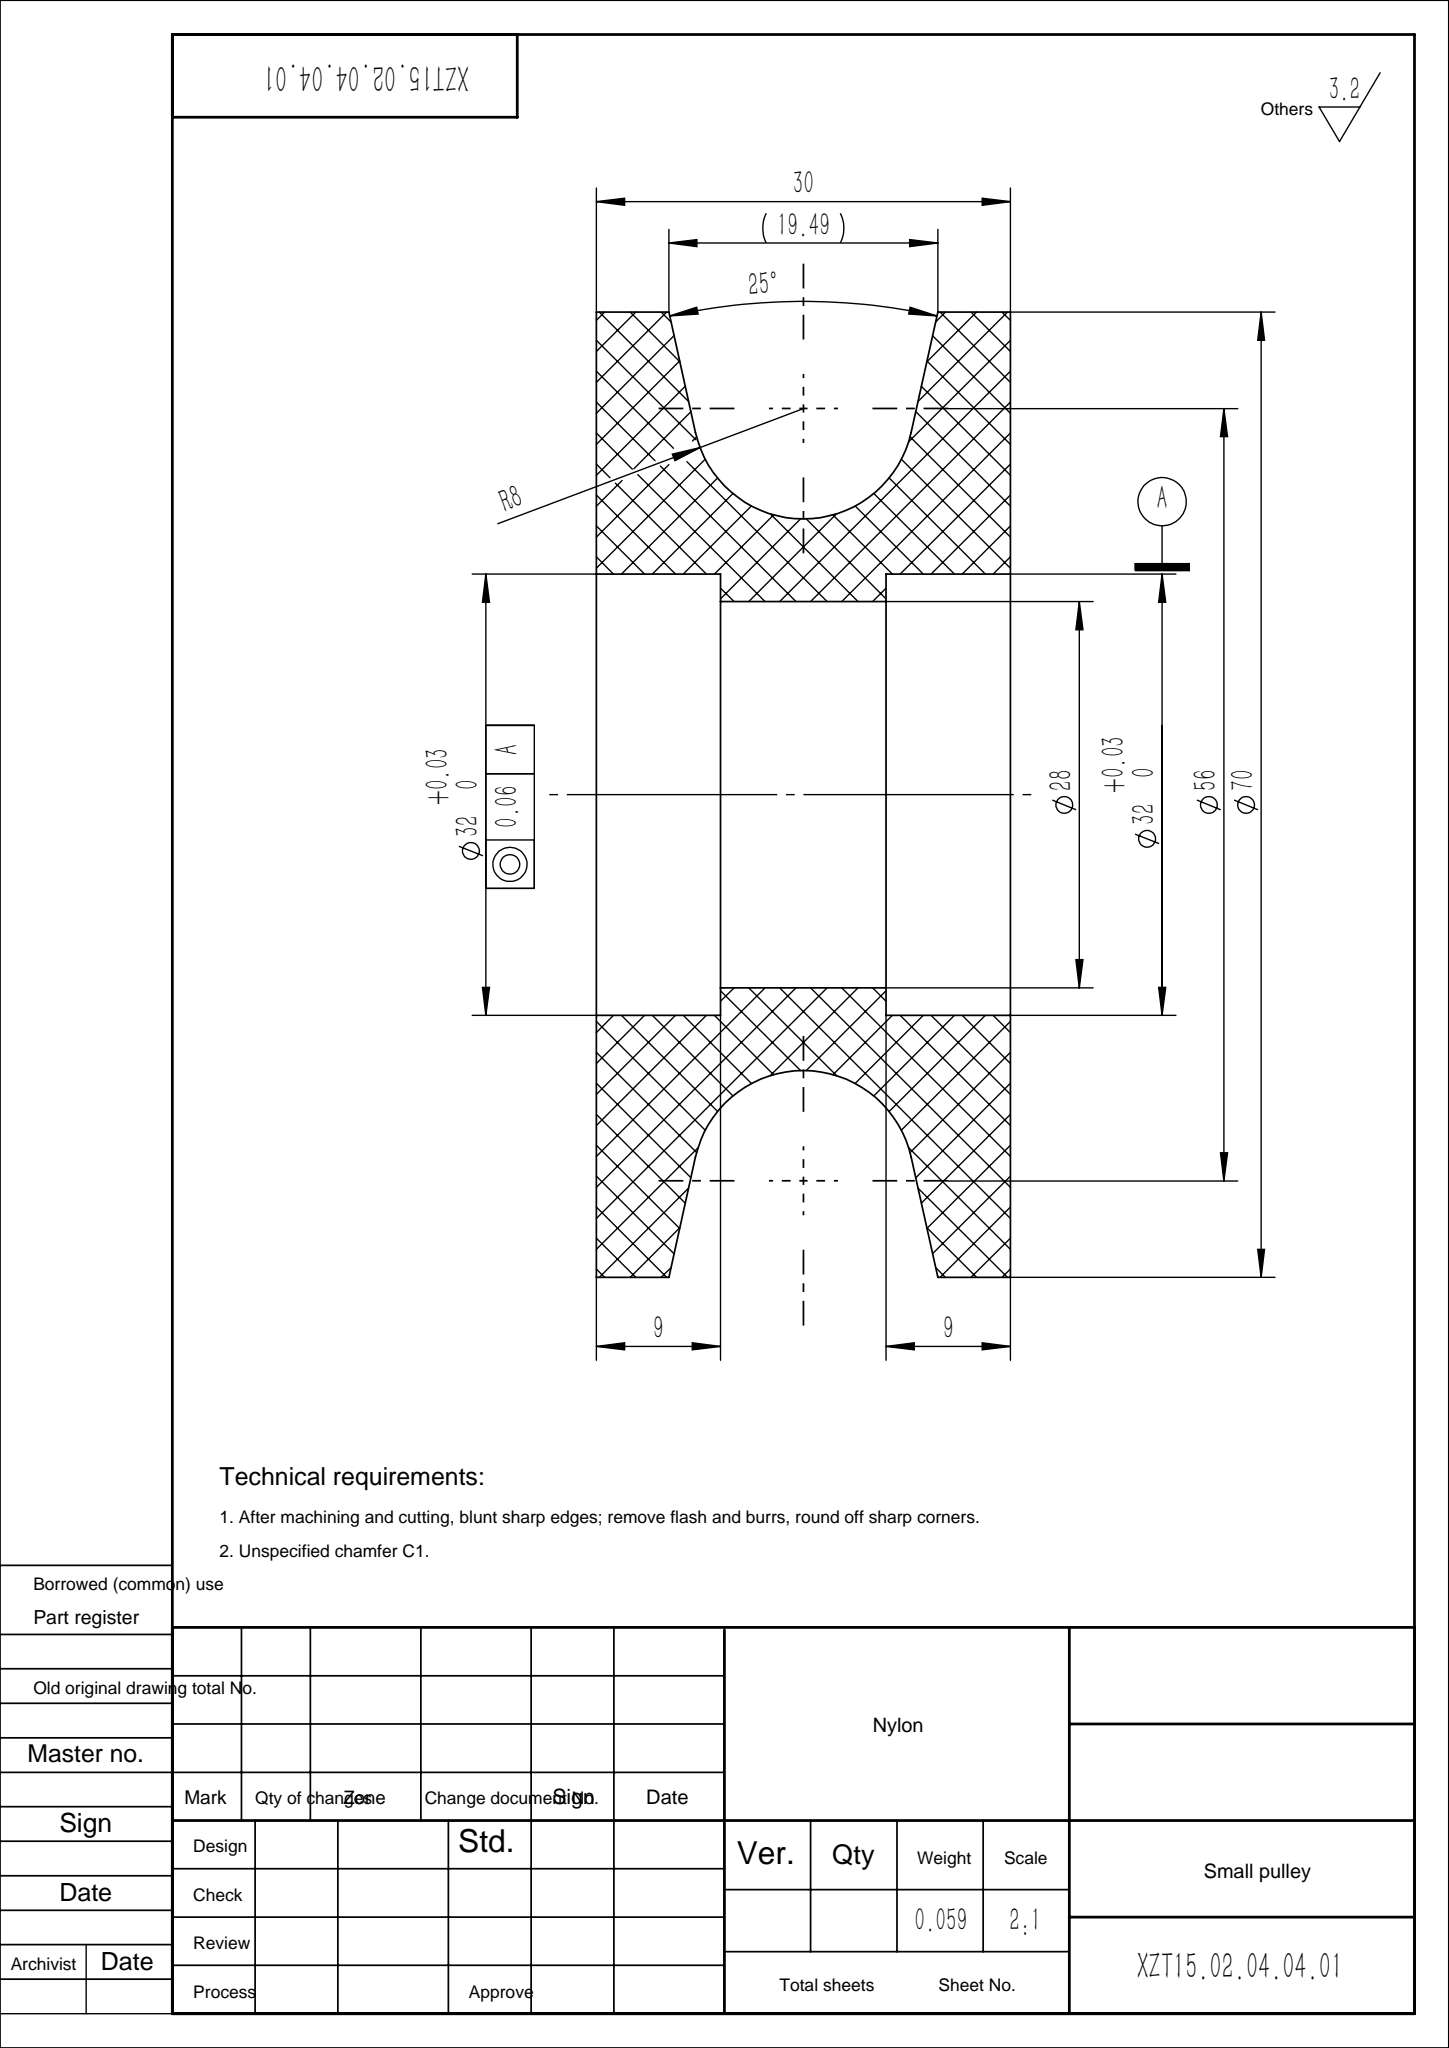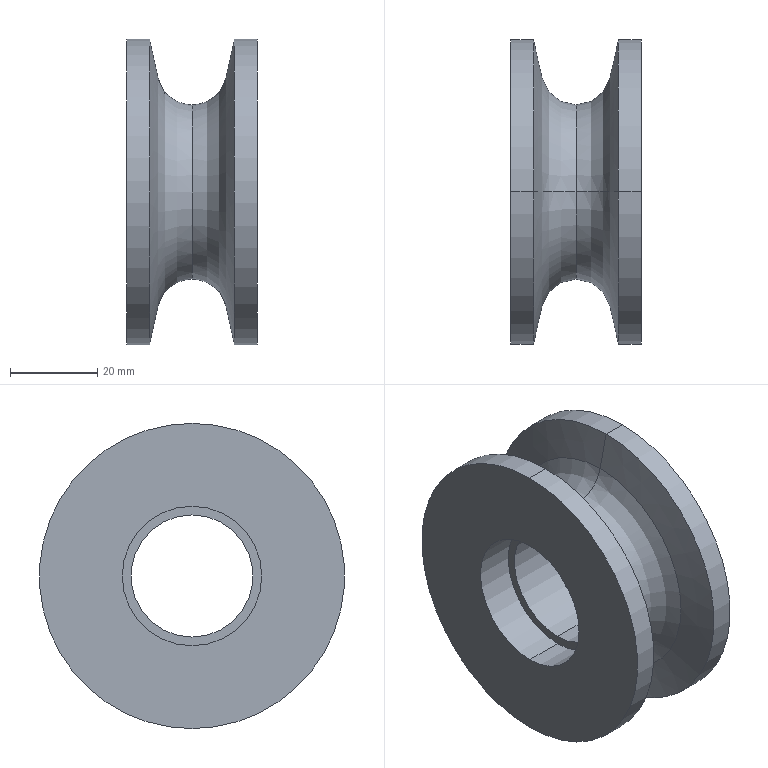Part | SolidWorks | features Revolution 1 | 1 solid | 22 faces | box 30 x 70 x 70 mm | volume 53072 mm3 | cylinder 10 | torus 4 | cone 4 | plane 4 | commonest cylinder face diameters 32 x4 70 x4 28 x2
STEP:
#1=CARTESIAN_POINT('',(-7.81,0.,26.268));
#2=VERTEX_POINT('',#1);
#3=CARTESIAN_POINT('',(0.,0.,20.));
#4=VERTEX_POINT('',#3);
#5=CARTESIAN_POINT('',(0.,0.,28.));
#6=DIRECTION('',(0.,-1.,0.));
#7=DIRECTION('',(0.,0.,-1.));
#8=AXIS2_PLACEMENT_3D('',#5,#6,#7);
#9=CIRCLE('',#8,8.);
#10=EDGE_CURVE('',#2,#4,#9,.T.);
#11=ORIENTED_EDGE('',*,*,#10,.T.);
#12=CARTESIAN_POINT('',(0.,0.,-20.));
#13=VERTEX_POINT('',#12);
#14=CARTESIAN_POINT('',(0.,0.,0.));
#15=DIRECTION('',(-1.,0.,0.));
#16=DIRECTION('',(0.,0.,1.));
#17=AXIS2_PLACEMENT_3D('',#14,#15,#16);
#18=CIRCLE('',#17,20.);
#19=EDGE_CURVE('',#4,#13,#18,.T.);
#20=ORIENTED_EDGE('',*,*,#19,.T.);
#21=CARTESIAN_POINT('',(-7.81,0.,-26.268));
#22=VERTEX_POINT('',#21);
#23=CARTESIAN_POINT('',(0.,0.,-28.));
#24=DIRECTION('',(0.,1.,0.));
#25=DIRECTION('',(0.,0.,1.));
#26=AXIS2_PLACEMENT_3D('',#23,#24,#25);
#27=CIRCLE('',#26,8.);
#28=EDGE_CURVE('',#22,#13,#27,.T.);
#29=ORIENTED_EDGE('',*,*,#28,.F.);
#30=CARTESIAN_POINT('',(-7.81,0.,0.));
#31=DIRECTION('',(-1.,0.,0.));
#32=DIRECTION('',(0.,0.,1.));
#33=AXIS2_PLACEMENT_3D('',#30,#31,#32);
#34=CIRCLE('',#33,26.268);
#35=EDGE_CURVE('',#2,#22,#34,.T.);
#36=ORIENTED_EDGE('',*,*,#35,.F.);
#37=EDGE_LOOP('',(#11,#20,#29,#36));
#38=FACE_OUTER_BOUND('',#37,.T.);
#39=CARTESIAN_POINT('',(0.,0.,0.));
#40=DIRECTION('',(-1.,0.,0.));
#41=DIRECTION('',(0.,0.,1.));
#42=AXIS2_PLACEMENT_3D('',#39,#40,#41);
#43=TOROIDAL_SURFACE('',#42,28.,8.);
#44=ADVANCED_FACE('',(#38),#43,.F.);
#45=ORIENTED_EDGE('',*,*,#28,.T.);
#46=CARTESIAN_POINT('',(0.,0.,0.));
#47=DIRECTION('',(-1.,0.,0.));
#48=DIRECTION('',(0.,0.,1.));
#49=AXIS2_PLACEMENT_3D('',#46,#47,#48);
#50=CIRCLE('',#49,20.);
#51=EDGE_CURVE('',#13,#4,#50,.T.);
#52=ORIENTED_EDGE('',*,*,#51,.T.);
#53=ORIENTED_EDGE('',*,*,#10,.F.);
#54=CARTESIAN_POINT('',(-7.81,0.,0.));
#55=DIRECTION('',(-1.,0.,0.));
#56=DIRECTION('',(0.,0.,1.));
#57=AXIS2_PLACEMENT_3D('',#54,#55,#56);
#58=CIRCLE('',#57,26.268);
#59=EDGE_CURVE('',#22,#2,#58,.T.);
#60=ORIENTED_EDGE('',*,*,#59,.F.);
#61=EDGE_LOOP('',(#45,#52,#53,#60));
#62=FACE_OUTER_BOUND('',#61,.T.);
#63=CARTESIAN_POINT('',(0.,0.,0.));
#64=DIRECTION('',(-1.,0.,0.));
#65=DIRECTION('',(0.,0.,1.));
#66=AXIS2_PLACEMENT_3D('',#63,#64,#65);
#67=TOROIDAL_SURFACE('',#66,28.,8.);
#68=ADVANCED_FACE('',(#62),#67,.F.);
#69=CARTESIAN_POINT('',(15.,0.,-16.));
#70=VERTEX_POINT('',#69);
#71=CARTESIAN_POINT('',(15.,0.,16.));
#72=VERTEX_POINT('',#71);
#73=CARTESIAN_POINT('',(15.,0.,0.));
#74=DIRECTION('',(-1.,0.,0.));
#75=DIRECTION('',(0.,0.,1.));
#76=AXIS2_PLACEMENT_3D('',#73,#74,#75);
#77=CIRCLE('',#76,16.);
#78=EDGE_CURVE('',#70,#72,#77,.T.);
#79=ORIENTED_EDGE('',*,*,#78,.F.);
#80=CARTESIAN_POINT('',(6.,0.,-16.));
#81=VERTEX_POINT('',#80);
#82=CARTESIAN_POINT('',(0.,0.,-16.));
#83=DIRECTION('',(-1.,0.,0.));
#84=VECTOR('',#83,1000.);
#85=LINE('',#82,#84);
#86=EDGE_CURVE('',#70,#81,#85,.T.);
#87=ORIENTED_EDGE('',*,*,#86,.T.);
#88=CARTESIAN_POINT('',(6.,0.,16.));
#89=VERTEX_POINT('',#88);
#90=CARTESIAN_POINT('',(6.,0.,0.));
#91=DIRECTION('',(-1.,0.,0.));
#92=DIRECTION('',(0.,0.,1.));
#93=AXIS2_PLACEMENT_3D('',#90,#91,#92);
#94=CIRCLE('',#93,16.);
#95=EDGE_CURVE('',#81,#89,#94,.T.);
#96=ORIENTED_EDGE('',*,*,#95,.T.);
#97=CARTESIAN_POINT('',(0.,0.,16.));
#98=DIRECTION('',(-1.,0.,0.));
#99=VECTOR('',#98,1000.);
#100=LINE('',#97,#99);
#101=EDGE_CURVE('',#72,#89,#100,.T.);
#102=ORIENTED_EDGE('',*,*,#101,.F.);
#103=EDGE_LOOP('',(#79,#87,#96,#102));
#104=FACE_OUTER_BOUND('',#103,.T.);
#105=CARTESIAN_POINT('',(0.,0.,0.));
#106=DIRECTION('',(-1.,0.,0.));
#107=DIRECTION('',(0.,0.,1.));
#108=AXIS2_PLACEMENT_3D('',#105,#106,#107);
#109=CYLINDRICAL_SURFACE('',#108,16.);
#110=ADVANCED_FACE('',(#104),#109,.F.);
#111=CARTESIAN_POINT('',(15.,0.,35.));
#112=VERTEX_POINT('',#111);
#113=CARTESIAN_POINT('',(15.,0.,-35.));
#114=VERTEX_POINT('',#113);
#115=CARTESIAN_POINT('',(15.,0.,0.));
#116=DIRECTION('',(-1.,0.,0.));
#117=DIRECTION('',(0.,0.,1.));
#118=AXIS2_PLACEMENT_3D('',#115,#116,#117);
#119=CIRCLE('',#118,35.);
#120=EDGE_CURVE('',#112,#114,#119,.T.);
#121=ORIENTED_EDGE('',*,*,#120,.T.);
#122=CARTESIAN_POINT('',(9.746,0.,-35.));
#123=VERTEX_POINT('',#122);
#124=CARTESIAN_POINT('',(0.,0.,-35.));
#125=DIRECTION('',(-1.,0.,0.));
#126=VECTOR('',#125,1000.);
#127=LINE('',#124,#126);
#128=EDGE_CURVE('',#114,#123,#127,.T.);
#129=ORIENTED_EDGE('',*,*,#128,.T.);
#130=CARTESIAN_POINT('',(9.746,0.,35.));
#131=VERTEX_POINT('',#130);
#132=CARTESIAN_POINT('',(9.746,0.,0.));
#133=DIRECTION('',(-1.,0.,0.));
#134=DIRECTION('',(0.,0.,1.));
#135=AXIS2_PLACEMENT_3D('',#132,#133,#134);
#136=CIRCLE('',#135,35.);
#137=EDGE_CURVE('',#131,#123,#136,.T.);
#138=ORIENTED_EDGE('',*,*,#137,.F.);
#139=CARTESIAN_POINT('',(0.,0.,35.));
#140=DIRECTION('',(-1.,0.,0.));
#141=VECTOR('',#140,1000.);
#142=LINE('',#139,#141);
#143=EDGE_CURVE('',#112,#131,#142,.T.);
#144=ORIENTED_EDGE('',*,*,#143,.F.);
#145=EDGE_LOOP('',(#121,#129,#138,#144));
#146=FACE_OUTER_BOUND('',#145,.T.);
#147=CARTESIAN_POINT('',(0.,0.,0.));
#148=DIRECTION('',(-1.,0.,0.));
#149=DIRECTION('',(0.,0.,1.));
#150=AXIS2_PLACEMENT_3D('',#147,#148,#149);
#151=CYLINDRICAL_SURFACE('',#150,35.);
#152=ADVANCED_FACE('',(#146),#151,.T.);
#153=CARTESIAN_POINT('',(7.81,0.,26.268));
#154=VERTEX_POINT('',#153);
#155=CARTESIAN_POINT('',(7.81,0.,-26.268));
#156=VERTEX_POINT('',#155);
#157=CARTESIAN_POINT('',(7.81,0.,0.));
#158=DIRECTION('',(-1.,0.,0.));
#159=DIRECTION('',(0.,0.,1.));
#160=AXIS2_PLACEMENT_3D('',#157,#158,#159);
#161=CIRCLE('',#160,26.268);
#162=EDGE_CURVE('',#154,#156,#161,.T.);
#163=ORIENTED_EDGE('',*,*,#162,.F.);
#164=CARTESIAN_POINT('',(9.746,0.,35.));
#165=DIRECTION('',(0.2164,0.,0.9763));
#166=VECTOR('',#165,1000.);
#167=LINE('',#164,#166);
#168=EDGE_CURVE('',#154,#131,#167,.T.);
#169=ORIENTED_EDGE('',*,*,#168,.T.);
#170=ORIENTED_EDGE('',*,*,#137,.T.);
#171=CARTESIAN_POINT('',(9.746,0.,-35.));
#172=DIRECTION('',(0.2164,0.,-0.9763));
#173=VECTOR('',#172,1000.);
#174=LINE('',#171,#173);
#175=EDGE_CURVE('',#156,#123,#174,.T.);
#176=ORIENTED_EDGE('',*,*,#175,.F.);
#177=EDGE_LOOP('',(#163,#169,#170,#176));
#178=FACE_OUTER_BOUND('',#177,.T.);
#179=CARTESIAN_POINT('',(9.746,0.,0.));
#180=DIRECTION('',(1.,0.,0.));
#181=DIRECTION('',(0.,0.,-1.));
#182=AXIS2_PLACEMENT_3D('',#179,#180,#181);
#183=CONICAL_SURFACE('',#182,35.,1.353);
#184=ADVANCED_FACE('',(#178),#183,.T.);
#185=ORIENTED_EDGE('',*,*,#51,.F.);
#186=CARTESIAN_POINT('',(0.,0.,-28.));
#187=DIRECTION('',(0.,1.,0.));
#188=DIRECTION('',(0.,0.,1.));
#189=AXIS2_PLACEMENT_3D('',#186,#187,#188);
#190=CIRCLE('',#189,8.);
#191=EDGE_CURVE('',#13,#156,#190,.T.);
#192=ORIENTED_EDGE('',*,*,#191,.T.);
#193=CARTESIAN_POINT('',(7.81,0.,0.));
#194=DIRECTION('',(-1.,0.,0.));
#195=DIRECTION('',(0.,0.,1.));
#196=AXIS2_PLACEMENT_3D('',#193,#194,#195);
#197=CIRCLE('',#196,26.268);
#198=EDGE_CURVE('',#156,#154,#197,.T.);
#199=ORIENTED_EDGE('',*,*,#198,.T.);
#200=CARTESIAN_POINT('',(0.,0.,28.));
#201=DIRECTION('',(0.,-1.,0.));
#202=DIRECTION('',(0.,0.,-1.));
#203=AXIS2_PLACEMENT_3D('',#200,#201,#202);
#204=CIRCLE('',#203,8.);
#205=EDGE_CURVE('',#4,#154,#204,.T.);
#206=ORIENTED_EDGE('',*,*,#205,.F.);
#207=EDGE_LOOP('',(#185,#192,#199,#206));
#208=FACE_OUTER_BOUND('',#207,.T.);
#209=CARTESIAN_POINT('',(0.,0.,0.));
#210=DIRECTION('',(-1.,0.,0.));
#211=DIRECTION('',(0.,0.,1.));
#212=AXIS2_PLACEMENT_3D('',#209,#210,#211);
#213=TOROIDAL_SURFACE('',#212,28.,8.);
#214=ADVANCED_FACE('',(#208),#213,.F.);
#215=ORIENTED_EDGE('',*,*,#35,.T.);
#216=CARTESIAN_POINT('',(-9.746,0.,-35.));
#217=VERTEX_POINT('',#216);
#218=CARTESIAN_POINT('',(-7.81,0.,-26.268));
#219=DIRECTION('',(-0.2164,0.,-0.9763));
#220=VECTOR('',#219,1000.);
#221=LINE('',#218,#220);
#222=EDGE_CURVE('',#22,#217,#221,.T.);
#223=ORIENTED_EDGE('',*,*,#222,.T.);
#224=CARTESIAN_POINT('',(-9.746,0.,35.));
#225=VERTEX_POINT('',#224);
#226=CARTESIAN_POINT('',(-9.746,0.,0.));
#227=DIRECTION('',(-1.,0.,0.));
#228=DIRECTION('',(0.,0.,1.));
#229=AXIS2_PLACEMENT_3D('',#226,#227,#228);
#230=CIRCLE('',#229,35.);
#231=EDGE_CURVE('',#225,#217,#230,.T.);
#232=ORIENTED_EDGE('',*,*,#231,.F.);
#233=CARTESIAN_POINT('',(-7.81,0.,26.268));
#234=DIRECTION('',(-0.2164,0.,0.9763));
#235=VECTOR('',#234,1000.);
#236=LINE('',#233,#235);
#237=EDGE_CURVE('',#2,#225,#236,.T.);
#238=ORIENTED_EDGE('',*,*,#237,.F.);
#239=EDGE_LOOP('',(#215,#223,#232,#238));
#240=FACE_OUTER_BOUND('',#239,.T.);
#241=CARTESIAN_POINT('',(-7.81,0.,0.));
#242=DIRECTION('',(-1.,0.,0.));
#243=DIRECTION('',(0.,0.,1.));
#244=AXIS2_PLACEMENT_3D('',#241,#242,#243);
#245=CONICAL_SURFACE('',#244,26.268,1.353);
#246=ADVANCED_FACE('',(#240),#245,.T.);
#247=ORIENTED_EDGE('',*,*,#231,.T.);
#248=CARTESIAN_POINT('',(-15.,0.,-35.));
#249=VERTEX_POINT('',#248);
#250=CARTESIAN_POINT('',(0.,0.,-35.));
#251=DIRECTION('',(-1.,0.,0.));
#252=VECTOR('',#251,1000.);
#253=LINE('',#250,#252);
#254=EDGE_CURVE('',#217,#249,#253,.T.);
#255=ORIENTED_EDGE('',*,*,#254,.T.);
#256=CARTESIAN_POINT('',(-15.,0.,35.));
#257=VERTEX_POINT('',#256);
#258=CARTESIAN_POINT('',(-15.,0.,0.));
#259=DIRECTION('',(-1.,0.,0.));
#260=DIRECTION('',(0.,0.,1.));
#261=AXIS2_PLACEMENT_3D('',#258,#259,#260);
#262=CIRCLE('',#261,35.);
#263=EDGE_CURVE('',#257,#249,#262,.T.);
#264=ORIENTED_EDGE('',*,*,#263,.F.);
#265=CARTESIAN_POINT('',(0.,0.,35.));
#266=DIRECTION('',(-1.,0.,0.));
#267=VECTOR('',#266,1000.);
#268=LINE('',#265,#267);
#269=EDGE_CURVE('',#225,#257,#268,.T.);
#270=ORIENTED_EDGE('',*,*,#269,.F.);
#271=EDGE_LOOP('',(#247,#255,#264,#270));
#272=FACE_OUTER_BOUND('',#271,.T.);
#273=CARTESIAN_POINT('',(0.,0.,0.));
#274=DIRECTION('',(-1.,0.,0.));
#275=DIRECTION('',(0.,0.,1.));
#276=AXIS2_PLACEMENT_3D('',#273,#274,#275);
#277=CYLINDRICAL_SURFACE('',#276,35.);
#278=ADVANCED_FACE('',(#272),#277,.T.);
#279=CARTESIAN_POINT('',(-6.,0.,-16.));
#280=VERTEX_POINT('',#279);
#281=CARTESIAN_POINT('',(-6.,0.,16.));
#282=VERTEX_POINT('',#281);
#283=CARTESIAN_POINT('',(-6.,0.,0.));
#284=DIRECTION('',(-1.,0.,0.));
#285=DIRECTION('',(0.,0.,1.));
#286=AXIS2_PLACEMENT_3D('',#283,#284,#285);
#287=CIRCLE('',#286,16.);
#288=EDGE_CURVE('',#280,#282,#287,.T.);
#289=ORIENTED_EDGE('',*,*,#288,.F.);
#290=CARTESIAN_POINT('',(-15.,0.,-16.));
#291=VERTEX_POINT('',#290);
#292=CARTESIAN_POINT('',(0.,0.,-16.));
#293=DIRECTION('',(-1.,0.,0.));
#294=VECTOR('',#293,1000.);
#295=LINE('',#292,#294);
#296=EDGE_CURVE('',#280,#291,#295,.T.);
#297=ORIENTED_EDGE('',*,*,#296,.T.);
#298=CARTESIAN_POINT('',(-15.,0.,16.));
#299=VERTEX_POINT('',#298);
#300=CARTESIAN_POINT('',(-15.,0.,0.));
#301=DIRECTION('',(-1.,0.,0.));
#302=DIRECTION('',(0.,0.,1.));
#303=AXIS2_PLACEMENT_3D('',#300,#301,#302);
#304=CIRCLE('',#303,16.);
#305=EDGE_CURVE('',#291,#299,#304,.T.);
#306=ORIENTED_EDGE('',*,*,#305,.T.);
#307=CARTESIAN_POINT('',(0.,0.,16.));
#308=DIRECTION('',(-1.,0.,0.));
#309=VECTOR('',#308,1000.);
#310=LINE('',#307,#309);
#311=EDGE_CURVE('',#282,#299,#310,.T.);
#312=ORIENTED_EDGE('',*,*,#311,.F.);
#313=EDGE_LOOP('',(#289,#297,#306,#312));
#314=FACE_OUTER_BOUND('',#313,.T.);
#315=CARTESIAN_POINT('',(0.,0.,0.));
#316=DIRECTION('',(-1.,0.,0.));
#317=DIRECTION('',(0.,0.,1.));
#318=AXIS2_PLACEMENT_3D('',#315,#316,#317);
#319=CYLINDRICAL_SURFACE('',#318,16.);
#320=ADVANCED_FACE('',(#314),#319,.F.);
#321=CARTESIAN_POINT('',(6.,0.,-14.));
#322=VERTEX_POINT('',#321);
#323=CARTESIAN_POINT('',(6.,0.,14.));
#324=VERTEX_POINT('',#323);
#325=CARTESIAN_POINT('',(6.,0.,0.));
#326=DIRECTION('',(-1.,0.,0.));
#327=DIRECTION('',(0.,0.,1.));
#328=AXIS2_PLACEMENT_3D('',#325,#326,#327);
#329=CIRCLE('',#328,14.);
#330=EDGE_CURVE('',#322,#324,#329,.T.);
#331=ORIENTED_EDGE('',*,*,#330,.F.);
#332=CARTESIAN_POINT('',(-6.,0.,-14.));
#333=VERTEX_POINT('',#332);
#334=CARTESIAN_POINT('',(0.,0.,-14.));
#335=DIRECTION('',(-1.,0.,0.));
#336=VECTOR('',#335,1000.);
#337=LINE('',#334,#336);
#338=EDGE_CURVE('',#322,#333,#337,.T.);
#339=ORIENTED_EDGE('',*,*,#338,.T.);
#340=CARTESIAN_POINT('',(-6.,0.,14.));
#341=VERTEX_POINT('',#340);
#342=CARTESIAN_POINT('',(-6.,0.,0.));
#343=DIRECTION('',(-1.,0.,0.));
#344=DIRECTION('',(0.,0.,1.));
#345=AXIS2_PLACEMENT_3D('',#342,#343,#344);
#346=CIRCLE('',#345,14.);
#347=EDGE_CURVE('',#333,#341,#346,.T.);
#348=ORIENTED_EDGE('',*,*,#347,.T.);
#349=CARTESIAN_POINT('',(0.,0.,14.));
#350=DIRECTION('',(-1.,0.,0.));
#351=VECTOR('',#350,1000.);
#352=LINE('',#349,#351);
#353=EDGE_CURVE('',#324,#341,#352,.T.);
#354=ORIENTED_EDGE('',*,*,#353,.F.);
#355=EDGE_LOOP('',(#331,#339,#348,#354));
#356=FACE_OUTER_BOUND('',#355,.T.);
#357=CARTESIAN_POINT('',(0.,0.,0.));
#358=DIRECTION('',(-1.,0.,0.));
#359=DIRECTION('',(0.,0.,1.));
#360=AXIS2_PLACEMENT_3D('',#357,#358,#359);
#361=CYLINDRICAL_SURFACE('',#360,14.);
#362=ADVANCED_FACE('',(#356),#361,.F.);
#363=CARTESIAN_POINT('',(6.,0.,0.));
#364=DIRECTION('',(-1.,0.,0.));
#365=DIRECTION('',(0.,0.,1.));
#366=AXIS2_PLACEMENT_3D('',#363,#364,#365);
#367=CIRCLE('',#366,16.);
#368=EDGE_CURVE('',#89,#81,#367,.T.);
#369=ORIENTED_EDGE('',*,*,#368,.F.);
#370=ORIENTED_EDGE('',*,*,#95,.F.);
#371=EDGE_LOOP('',(#369,#370));
#372=FACE_OUTER_BOUND('',#371,.T.);
#373=CARTESIAN_POINT('',(6.,0.,0.));
#374=DIRECTION('',(-1.,0.,0.));
#375=DIRECTION('',(0.,0.,1.));
#376=AXIS2_PLACEMENT_3D('',#373,#374,#375);
#377=CIRCLE('',#376,14.);
#378=EDGE_CURVE('',#324,#322,#377,.T.);
#379=ORIENTED_EDGE('',*,*,#378,.T.);
#380=ORIENTED_EDGE('',*,*,#330,.T.);
#381=EDGE_LOOP('',(#379,#380));
#382=FACE_BOUND('',#381,.T.);
#383=CARTESIAN_POINT('',(6.,14.,0.));
#384=DIRECTION('',(-1.,0.,0.));
#385=DIRECTION('',(0.,0.,1.));
#386=AXIS2_PLACEMENT_3D('',#383,#384,#385);
#387=PLANE('',#386);
#388=ADVANCED_FACE('',(#372,#382),#387,.F.);
#389=ORIENTED_EDGE('',*,*,#338,.F.);
#390=ORIENTED_EDGE('',*,*,#378,.F.);
#391=ORIENTED_EDGE('',*,*,#353,.T.);
#392=CARTESIAN_POINT('',(-6.,0.,0.));
#393=DIRECTION('',(-1.,0.,0.));
#394=DIRECTION('',(0.,0.,1.));
#395=AXIS2_PLACEMENT_3D('',#392,#393,#394);
#396=CIRCLE('',#395,14.);
#397=EDGE_CURVE('',#341,#333,#396,.T.);
#398=ORIENTED_EDGE('',*,*,#397,.T.);
#399=EDGE_LOOP('',(#389,#390,#391,#398));
#400=FACE_OUTER_BOUND('',#399,.T.);
#401=CARTESIAN_POINT('',(0.,0.,0.));
#402=DIRECTION('',(-1.,0.,0.));
#403=DIRECTION('',(0.,0.,1.));
#404=AXIS2_PLACEMENT_3D('',#401,#402,#403);
#405=CYLINDRICAL_SURFACE('',#404,14.);
#406=ADVANCED_FACE('',(#400),#405,.F.);
#407=ORIENTED_EDGE('',*,*,#397,.F.);
#408=ORIENTED_EDGE('',*,*,#347,.F.);
#409=EDGE_LOOP('',(#407,#408));
#410=FACE_BOUND('',#409,.T.);
#411=CARTESIAN_POINT('',(-6.,0.,0.));
#412=DIRECTION('',(-1.,0.,0.));
#413=DIRECTION('',(0.,0.,1.));
#414=AXIS2_PLACEMENT_3D('',#411,#412,#413);
#415=CIRCLE('',#414,16.);
#416=EDGE_CURVE('',#282,#280,#415,.T.);
#417=ORIENTED_EDGE('',*,*,#416,.T.);
#418=ORIENTED_EDGE('',*,*,#288,.T.);
#419=EDGE_LOOP('',(#417,#418));
#420=FACE_OUTER_BOUND('',#419,.T.);
#421=CARTESIAN_POINT('',(-6.,14.,0.));
#422=DIRECTION('',(1.,0.,0.));
#423=DIRECTION('',(0.,0.,-1.));
#424=AXIS2_PLACEMENT_3D('',#421,#422,#423);
#425=PLANE('',#424);
#426=ADVANCED_FACE('',(#410,#420),#425,.F.);
#427=ORIENTED_EDGE('',*,*,#296,.F.);
#428=ORIENTED_EDGE('',*,*,#416,.F.);
#429=ORIENTED_EDGE('',*,*,#311,.T.);
#430=CARTESIAN_POINT('',(-15.,0.,0.));
#431=DIRECTION('',(-1.,0.,0.));
#432=DIRECTION('',(0.,0.,1.));
#433=AXIS2_PLACEMENT_3D('',#430,#431,#432);
#434=CIRCLE('',#433,16.);
#435=EDGE_CURVE('',#299,#291,#434,.T.);
#436=ORIENTED_EDGE('',*,*,#435,.T.);
#437=EDGE_LOOP('',(#427,#428,#429,#436));
#438=FACE_OUTER_BOUND('',#437,.T.);
#439=CARTESIAN_POINT('',(0.,0.,0.));
#440=DIRECTION('',(-1.,0.,0.));
#441=DIRECTION('',(0.,0.,1.));
#442=AXIS2_PLACEMENT_3D('',#439,#440,#441);
#443=CYLINDRICAL_SURFACE('',#442,16.);
#444=ADVANCED_FACE('',(#438),#443,.F.);
#445=ORIENTED_EDGE('',*,*,#435,.F.);
#446=ORIENTED_EDGE('',*,*,#305,.F.);
#447=EDGE_LOOP('',(#445,#446));
#448=FACE_BOUND('',#447,.T.);
#449=ORIENTED_EDGE('',*,*,#263,.T.);
#450=CARTESIAN_POINT('',(-15.,0.,0.));
#451=DIRECTION('',(-1.,0.,0.));
#452=DIRECTION('',(0.,0.,1.));
#453=AXIS2_PLACEMENT_3D('',#450,#451,#452);
#454=CIRCLE('',#453,35.);
#455=EDGE_CURVE('',#249,#257,#454,.T.);
#456=ORIENTED_EDGE('',*,*,#455,.T.);
#457=EDGE_LOOP('',(#449,#456));
#458=FACE_OUTER_BOUND('',#457,.T.);
#459=CARTESIAN_POINT('',(-15.,16.,0.));
#460=DIRECTION('',(1.,0.,0.));
#461=DIRECTION('',(0.,0.,-1.));
#462=AXIS2_PLACEMENT_3D('',#459,#460,#461);
#463=PLANE('',#462);
#464=ADVANCED_FACE('',(#448,#458),#463,.F.);
#465=ORIENTED_EDGE('',*,*,#254,.F.);
#466=CARTESIAN_POINT('',(-9.746,0.,0.));
#467=DIRECTION('',(-1.,0.,0.));
#468=DIRECTION('',(0.,0.,1.));
#469=AXIS2_PLACEMENT_3D('',#466,#467,#468);
#470=CIRCLE('',#469,35.);
#471=EDGE_CURVE('',#217,#225,#470,.T.);
#472=ORIENTED_EDGE('',*,*,#471,.T.);
#473=ORIENTED_EDGE('',*,*,#269,.T.);
#474=ORIENTED_EDGE('',*,*,#455,.F.);
#475=EDGE_LOOP('',(#465,#472,#473,#474));
#476=FACE_OUTER_BOUND('',#475,.T.);
#477=CARTESIAN_POINT('',(0.,0.,0.));
#478=DIRECTION('',(-1.,0.,0.));
#479=DIRECTION('',(0.,0.,1.));
#480=AXIS2_PLACEMENT_3D('',#477,#478,#479);
#481=CYLINDRICAL_SURFACE('',#480,35.);
#482=ADVANCED_FACE('',(#476),#481,.T.);
#483=ORIENTED_EDGE('',*,*,#222,.F.);
#484=ORIENTED_EDGE('',*,*,#59,.T.);
#485=ORIENTED_EDGE('',*,*,#237,.T.);
#486=ORIENTED_EDGE('',*,*,#471,.F.);
#487=EDGE_LOOP('',(#483,#484,#485,#486));
#488=FACE_OUTER_BOUND('',#487,.T.);
#489=CARTESIAN_POINT('',(-7.81,0.,0.));
#490=DIRECTION('',(-1.,0.,0.));
#491=DIRECTION('',(0.,0.,1.));
#492=AXIS2_PLACEMENT_3D('',#489,#490,#491);
#493=CONICAL_SURFACE('',#492,26.268,1.353);
#494=ADVANCED_FACE('',(#488),#493,.T.);
#495=ORIENTED_EDGE('',*,*,#19,.F.);
#496=ORIENTED_EDGE('',*,*,#205,.T.);
#497=ORIENTED_EDGE('',*,*,#162,.T.);
#498=ORIENTED_EDGE('',*,*,#191,.F.);
#499=EDGE_LOOP('',(#495,#496,#497,#498));
#500=FACE_OUTER_BOUND('',#499,.T.);
#501=CARTESIAN_POINT('',(0.,0.,0.));
#502=DIRECTION('',(-1.,0.,0.));
#503=DIRECTION('',(0.,0.,1.));
#504=AXIS2_PLACEMENT_3D('',#501,#502,#503);
#505=TOROIDAL_SURFACE('',#504,28.,8.);
#506=ADVANCED_FACE('',(#500),#505,.F.);
#507=ORIENTED_EDGE('',*,*,#168,.F.);
#508=ORIENTED_EDGE('',*,*,#198,.F.);
#509=ORIENTED_EDGE('',*,*,#175,.T.);
#510=CARTESIAN_POINT('',(9.746,0.,0.));
#511=DIRECTION('',(-1.,0.,0.));
#512=DIRECTION('',(0.,0.,1.));
#513=AXIS2_PLACEMENT_3D('',#510,#511,#512);
#514=CIRCLE('',#513,35.);
#515=EDGE_CURVE('',#123,#131,#514,.T.);
#516=ORIENTED_EDGE('',*,*,#515,.T.);
#517=EDGE_LOOP('',(#507,#508,#509,#516));
#518=FACE_OUTER_BOUND('',#517,.T.);
#519=CARTESIAN_POINT('',(9.746,0.,0.));
#520=DIRECTION('',(1.,0.,0.));
#521=DIRECTION('',(0.,0.,-1.));
#522=AXIS2_PLACEMENT_3D('',#519,#520,#521);
#523=CONICAL_SURFACE('',#522,35.,1.353);
#524=ADVANCED_FACE('',(#518),#523,.T.);
#525=ORIENTED_EDGE('',*,*,#128,.F.);
#526=CARTESIAN_POINT('',(15.,0.,0.));
#527=DIRECTION('',(-1.,0.,0.));
#528=DIRECTION('',(0.,0.,1.));
#529=AXIS2_PLACEMENT_3D('',#526,#527,#528);
#530=CIRCLE('',#529,35.);
#531=EDGE_CURVE('',#114,#112,#530,.T.);
#532=ORIENTED_EDGE('',*,*,#531,.T.);
#533=ORIENTED_EDGE('',*,*,#143,.T.);
#534=ORIENTED_EDGE('',*,*,#515,.F.);
#535=EDGE_LOOP('',(#525,#532,#533,#534));
#536=FACE_OUTER_BOUND('',#535,.T.);
#537=CARTESIAN_POINT('',(0.,0.,0.));
#538=DIRECTION('',(-1.,0.,0.));
#539=DIRECTION('',(0.,0.,1.));
#540=AXIS2_PLACEMENT_3D('',#537,#538,#539);
#541=CYLINDRICAL_SURFACE('',#540,35.);
#542=ADVANCED_FACE('',(#536),#541,.T.);
#543=ORIENTED_EDGE('',*,*,#120,.F.);
#544=ORIENTED_EDGE('',*,*,#531,.F.);
#545=EDGE_LOOP('',(#543,#544));
#546=FACE_OUTER_BOUND('',#545,.T.);
#547=CARTESIAN_POINT('',(15.,0.,0.));
#548=DIRECTION('',(-1.,0.,0.));
#549=DIRECTION('',(0.,0.,1.));
#550=AXIS2_PLACEMENT_3D('',#547,#548,#549);
#551=CIRCLE('',#550,16.);
#552=EDGE_CURVE('',#72,#70,#551,.T.);
#553=ORIENTED_EDGE('',*,*,#552,.T.);
#554=ORIENTED_EDGE('',*,*,#78,.T.);
#555=EDGE_LOOP('',(#553,#554));
#556=FACE_BOUND('',#555,.T.);
#557=CARTESIAN_POINT('',(15.,16.,0.));
#558=DIRECTION('',(-1.,0.,0.));
#559=DIRECTION('',(0.,0.,1.));
#560=AXIS2_PLACEMENT_3D('',#557,#558,#559);
#561=PLANE('',#560);
#562=ADVANCED_FACE('',(#546,#556),#561,.F.);
#563=ORIENTED_EDGE('',*,*,#86,.F.);
#564=ORIENTED_EDGE('',*,*,#552,.F.);
#565=ORIENTED_EDGE('',*,*,#101,.T.);
#566=ORIENTED_EDGE('',*,*,#368,.T.);
#567=EDGE_LOOP('',(#563,#564,#565,#566));
#568=FACE_OUTER_BOUND('',#567,.T.);
#569=CARTESIAN_POINT('',(0.,0.,0.));
#570=DIRECTION('',(-1.,0.,0.));
#571=DIRECTION('',(0.,0.,1.));
#572=AXIS2_PLACEMENT_3D('',#569,#570,#571);
#573=CYLINDRICAL_SURFACE('',#572,16.);
#574=ADVANCED_FACE('',(#568),#573,.F.);
#575=CLOSED_SHELL('',(#44,#68,#110,#152,#184,#214,#246,#278,#320,#362,#388,#406,#426,#444,#464,#482,#494,#506,#524,#542,#562,#574));
#576=MANIFOLD_SOLID_BREP('',#575);
#577=CARTESIAN_POINT('',(0.,0.,0.));
#578=DIRECTION('',(0.,0.,1.));
#579=DIRECTION('',(1.,0.,0.));
#580=AXIS2_PLACEMENT_3D('',#577,#578,#579);
#581=(LENGTH_UNIT()NAMED_UNIT(*)SI_UNIT(.MILLI.,.METRE.));
#582=UNCERTAINTY_MEASURE_WITH_UNIT(LENGTH_MEASURE(0.00001),#581,'','');
#583=(NAMED_UNIT(*)PLANE_ANGLE_UNIT()SI_UNIT($,.RADIAN.));
#584=(NAMED_UNIT(*)SI_UNIT($,.STERADIAN.)SOLID_ANGLE_UNIT());
#585=(GEOMETRIC_REPRESENTATION_CONTEXT(3)GLOBAL_UNCERTAINTY_ASSIGNED_CONTEXT((#582))GLOBAL_UNIT_ASSIGNED_CONTEXT((#581,#583,#584))REPRESENTATION_CONTEXT('',''));
#586=ADVANCED_BREP_SHAPE_REPRESENTATION('',(#576,#580),#585);